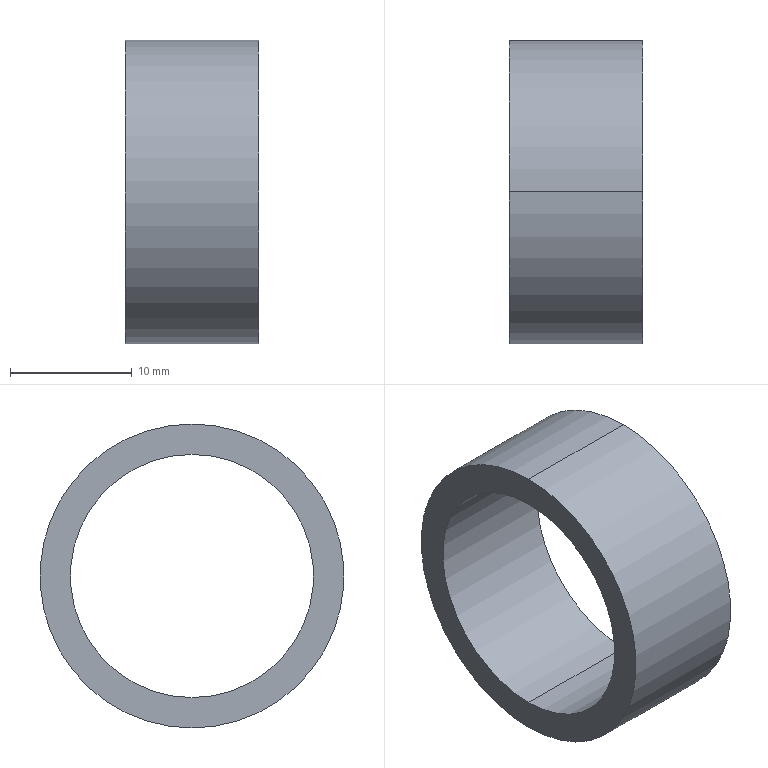Part | STEP file | 0244_Z_002_BSW20_2 | 1 solid | 6 faces | box 11 x 25 x 25 mm | volume 1944 mm3 | cylinder 4 | plane 2 | commonest cylinder face diameters 20 x2 25 x2
STEP:
#1=CARTESIAN_POINT('',(0.,0.,0.));
#2=DIRECTION('',(0.,0.,1.));
#3=DIRECTION('',(1.,0.,0.));
#4=AXIS2_PLACEMENT_3D('',#1,#2,#3);
#5=CARTESIAN_POINT('',(17.,30.,-12.5));
#6=VERTEX_POINT('',#5);
#7=CARTESIAN_POINT('',(17.,30.,12.5));
#8=VERTEX_POINT('',#7);
#9=CARTESIAN_POINT('',(17.,30.,0.));
#10=DIRECTION('',(1.,0.,0.));
#11=DIRECTION('',(0.,0.,-1.));
#12=AXIS2_PLACEMENT_3D('',#9,#10,#11);
#13=CIRCLE('',#12,12.5);
#14=CARTESIAN_POINT('',(22.5,30.,0.));
#15=DIRECTION('',(1.,0.,0.));
#16=DIRECTION('',(0.,0.,-1.));
#17=AXIS2_PLACEMENT_3D('',#14,#15,#16);
#18=CYLINDRICAL_SURFACE('',#17,12.5);
#19=CARTESIAN_POINT('',(0.,-5.5));
#20=DIRECTION('',(1.,0.));
#21=VECTOR('',#20,1.);
#22=LINE('',#19,#21);
#23=(GEOMETRIC_REPRESENTATION_CONTEXT(2)PARAMETRIC_REPRESENTATION_CONTEXT()REPRESENTATION_CONTEXT('',''));
#24=DEFINITIONAL_REPRESENTATION('',(#22),#23);
#25=PCURVE('',#18,#24);
#26=CARTESIAN_POINT('',(17.,18.75,0.));
#27=DIRECTION('',(-1.,0.,0.));
#28=DIRECTION('',(0.,0.,1.));
#29=AXIS2_PLACEMENT_3D('',#26,#27,#28);
#30=PLANE('',#29);
#31=CARTESIAN_POINT('',(-12.5,11.25));
#32=CARTESIAN_POINT('',(-12.5,32.901));
#33=CARTESIAN_POINT('',(6.25,22.075));
#34=CARTESIAN_POINT('',(25.,11.25));
#35=CARTESIAN_POINT('',(6.25,0.4247));
#36=CARTESIAN_POINT('',(-12.5,-10.401));
#37=CARTESIAN_POINT('',(-12.5,11.25));
#38=(BOUNDED_CURVE()B_SPLINE_CURVE(2,(#31,#32,#33,#34,#35,#36,#37),.UNSPECIFIED.,.T.,.F.)B_SPLINE_CURVE_WITH_KNOTS((1,2,2,2,2,1),(-2.094,0.,2.094,4.189,6.283,8.378),.UNSPECIFIED.)CURVE()GEOMETRIC_REPRESENTATION_ITEM()RATIONAL_B_SPLINE_CURVE((1.,0.5,1.,0.5,1.,0.5,1.))REPRESENTATION_ITEM(''));
#39=(GEOMETRIC_REPRESENTATION_CONTEXT(2)PARAMETRIC_REPRESENTATION_CONTEXT()REPRESENTATION_CONTEXT('',''));
#40=DEFINITIONAL_REPRESENTATION('',(#38),#39);
#41=PCURVE('',#30,#40);
#42=SURFACE_CURVE('',#13,(#25,#41),.PCURVE_S1.);
#43=EDGE_CURVE('',#6,#8,#42,.T.);
#44=ORIENTED_EDGE('',*,*,#43,.T.);
#45=CARTESIAN_POINT('',(28.,30.,12.5));
#46=VERTEX_POINT('',#45);
#47=CARTESIAN_POINT('',(22.5,30.,12.5));
#48=DIRECTION('',(1.,0.,0.));
#49=VECTOR('',#48,1.);
#50=LINE('',#47,#49);
#51=CARTESIAN_POINT('',(3.142,0.));
#52=DIRECTION('',(0.,1.));
#53=VECTOR('',#52,1.);
#54=LINE('',#51,#53);
#55=(GEOMETRIC_REPRESENTATION_CONTEXT(2)PARAMETRIC_REPRESENTATION_CONTEXT()REPRESENTATION_CONTEXT('',''));
#56=DEFINITIONAL_REPRESENTATION('',(#54),#55);
#57=PCURVE('',#18,#56);
#58=CARTESIAN_POINT('',(22.5,30.,0.));
#59=DIRECTION('',(1.,0.,0.));
#60=DIRECTION('',(0.,0.,-1.));
#61=AXIS2_PLACEMENT_3D('',#58,#59,#60);
#62=CYLINDRICAL_SURFACE('',#61,12.5);
#63=CARTESIAN_POINT('',(3.142,0.));
#64=DIRECTION('',(0.,1.));
#65=VECTOR('',#64,1.);
#66=LINE('',#63,#65);
#67=(GEOMETRIC_REPRESENTATION_CONTEXT(2)PARAMETRIC_REPRESENTATION_CONTEXT()REPRESENTATION_CONTEXT('',''));
#68=DEFINITIONAL_REPRESENTATION('',(#66),#67);
#69=PCURVE('',#62,#68);
#70=SURFACE_CURVE('',#50,(#57,#69),.PCURVE_S1.);
#71=EDGE_CURVE('',#8,#46,#70,.T.);
#72=ORIENTED_EDGE('',*,*,#71,.T.);
#73=CARTESIAN_POINT('',(28.,30.,-12.5));
#74=VERTEX_POINT('',#73);
#75=CARTESIAN_POINT('',(28.,30.,0.));
#76=DIRECTION('',(-1.,0.,0.));
#77=DIRECTION('',(0.,0.,-1.));
#78=AXIS2_PLACEMENT_3D('',#75,#76,#77);
#79=CIRCLE('',#78,12.5);
#80=CARTESIAN_POINT('',(6.283,5.5));
#81=DIRECTION('',(-1.,0.));
#82=VECTOR('',#81,1.);
#83=LINE('',#80,#82);
#84=(GEOMETRIC_REPRESENTATION_CONTEXT(2)PARAMETRIC_REPRESENTATION_CONTEXT()REPRESENTATION_CONTEXT('',''));
#85=DEFINITIONAL_REPRESENTATION('',(#83),#84);
#86=PCURVE('',#18,#85);
#87=CARTESIAN_POINT('',(28.,18.75,0.));
#88=DIRECTION('',(1.,0.,0.));
#89=DIRECTION('',(0.,0.,-1.));
#90=AXIS2_PLACEMENT_3D('',#87,#88,#89);
#91=PLANE('',#90);
#92=CARTESIAN_POINT('',(12.5,11.25));
#93=CARTESIAN_POINT('',(12.5,-10.401));
#94=CARTESIAN_POINT('',(-6.25,0.4247));
#95=CARTESIAN_POINT('',(-25.,11.25));
#96=CARTESIAN_POINT('',(-6.25,22.075));
#97=CARTESIAN_POINT('',(12.5,32.901));
#98=CARTESIAN_POINT('',(12.5,11.25));
#99=(BOUNDED_CURVE()B_SPLINE_CURVE(2,(#92,#93,#94,#95,#96,#97,#98),.UNSPECIFIED.,.T.,.F.)B_SPLINE_CURVE_WITH_KNOTS((1,2,2,2,2,1),(-2.094,0.,2.094,4.189,6.283,8.378),.UNSPECIFIED.)CURVE()GEOMETRIC_REPRESENTATION_ITEM()RATIONAL_B_SPLINE_CURVE((1.,0.5,1.,0.5,1.,0.5,1.))REPRESENTATION_ITEM(''));
#100=(GEOMETRIC_REPRESENTATION_CONTEXT(2)PARAMETRIC_REPRESENTATION_CONTEXT()REPRESENTATION_CONTEXT('',''));
#101=DEFINITIONAL_REPRESENTATION('',(#99),#100);
#102=PCURVE('',#91,#101);
#103=SURFACE_CURVE('',#79,(#86,#102),.PCURVE_S1.);
#104=EDGE_CURVE('',#46,#74,#103,.T.);
#105=ORIENTED_EDGE('',*,*,#104,.T.);
#106=CARTESIAN_POINT('',(22.5,30.,-12.5));
#107=DIRECTION('',(1.,0.,0.));
#108=VECTOR('',#107,1.);
#109=LINE('',#106,#108);
#110=CARTESIAN_POINT('',(0.,0.));
#111=DIRECTION('',(0.,1.));
#112=VECTOR('',#111,1.);
#113=LINE('',#110,#112);
#114=(GEOMETRIC_REPRESENTATION_CONTEXT(2)PARAMETRIC_REPRESENTATION_CONTEXT()REPRESENTATION_CONTEXT('',''));
#115=DEFINITIONAL_REPRESENTATION('',(#113),#114);
#116=PCURVE('',#18,#115);
#117=CARTESIAN_POINT('',(6.283,0.));
#118=DIRECTION('',(0.,1.));
#119=VECTOR('',#118,1.);
#120=LINE('',#117,#119);
#121=(GEOMETRIC_REPRESENTATION_CONTEXT(2)PARAMETRIC_REPRESENTATION_CONTEXT()REPRESENTATION_CONTEXT('',''));
#122=DEFINITIONAL_REPRESENTATION('',(#120),#121);
#123=PCURVE('',#62,#122);
#124=SURFACE_CURVE('',#109,(#116,#123),.PCURVE_S1.);
#125=EDGE_CURVE('',#6,#74,#124,.T.);
#126=ORIENTED_EDGE('',*,*,#125,.F.);
#127=EDGE_LOOP('',(#44,#72,#105,#126));
#128=FACE_BOUND('',#127,.T.);
#129=ADVANCED_FACE('',(#128),#18,.T.);
#130=CARTESIAN_POINT('',(17.,30.,-10.));
#131=VERTEX_POINT('',#130);
#132=CARTESIAN_POINT('',(28.,30.,-10.));
#133=VERTEX_POINT('',#132);
#134=CARTESIAN_POINT('',(22.5,30.,-10.));
#135=DIRECTION('',(1.,0.,0.));
#136=VECTOR('',#135,1.);
#137=LINE('',#134,#136);
#138=CARTESIAN_POINT('',(22.5,30.,0.));
#139=DIRECTION('',(1.,0.,0.));
#140=DIRECTION('',(0.,0.,-1.));
#141=AXIS2_PLACEMENT_3D('',#138,#139,#140);
#142=CYLINDRICAL_SURFACE('',#141,10.);
#143=CARTESIAN_POINT('',(6.283,0.));
#144=DIRECTION('',(0.,1.));
#145=VECTOR('',#144,1.);
#146=LINE('',#143,#145);
#147=(GEOMETRIC_REPRESENTATION_CONTEXT(2)PARAMETRIC_REPRESENTATION_CONTEXT()REPRESENTATION_CONTEXT('',''));
#148=DEFINITIONAL_REPRESENTATION('',(#146),#147);
#149=PCURVE('',#142,#148);
#150=CARTESIAN_POINT('',(22.5,30.,0.));
#151=DIRECTION('',(1.,0.,0.));
#152=DIRECTION('',(0.,0.,-1.));
#153=AXIS2_PLACEMENT_3D('',#150,#151,#152);
#154=CYLINDRICAL_SURFACE('',#153,10.);
#155=CARTESIAN_POINT('',(0.,0.));
#156=DIRECTION('',(0.,1.));
#157=VECTOR('',#156,1.);
#158=LINE('',#155,#157);
#159=(GEOMETRIC_REPRESENTATION_CONTEXT(2)PARAMETRIC_REPRESENTATION_CONTEXT()REPRESENTATION_CONTEXT('',''));
#160=DEFINITIONAL_REPRESENTATION('',(#158),#159);
#161=PCURVE('',#154,#160);
#162=SURFACE_CURVE('',#137,(#149,#161),.PCURVE_S1.);
#163=EDGE_CURVE('',#131,#133,#162,.T.);
#164=ORIENTED_EDGE('',*,*,#163,.T.);
#165=CARTESIAN_POINT('',(28.,30.,10.));
#166=VERTEX_POINT('',#165);
#167=CARTESIAN_POINT('',(28.,30.,0.));
#168=DIRECTION('',(-1.,0.,0.));
#169=DIRECTION('',(0.,0.,-1.));
#170=AXIS2_PLACEMENT_3D('',#167,#168,#169);
#171=CIRCLE('',#170,10.);
#172=CARTESIAN_POINT('',(6.283,5.5));
#173=DIRECTION('',(-1.,0.));
#174=VECTOR('',#173,1.);
#175=LINE('',#172,#174);
#176=(GEOMETRIC_REPRESENTATION_CONTEXT(2)PARAMETRIC_REPRESENTATION_CONTEXT()REPRESENTATION_CONTEXT('',''));
#177=DEFINITIONAL_REPRESENTATION('',(#175),#176);
#178=PCURVE('',#142,#177);
#179=CARTESIAN_POINT('',(10.,11.25));
#180=CARTESIAN_POINT('',(10.,-6.071));
#181=CARTESIAN_POINT('',(-5.,2.59));
#182=CARTESIAN_POINT('',(-20.,11.25));
#183=CARTESIAN_POINT('',(-5.,19.91));
#184=CARTESIAN_POINT('',(10.,28.571));
#185=CARTESIAN_POINT('',(10.,11.25));
#186=(BOUNDED_CURVE()B_SPLINE_CURVE(2,(#179,#180,#181,#182,#183,#184,#185),.UNSPECIFIED.,.T.,.F.)B_SPLINE_CURVE_WITH_KNOTS((1,2,2,2,2,1),(-2.094,0.,2.094,4.189,6.283,8.378),.UNSPECIFIED.)CURVE()GEOMETRIC_REPRESENTATION_ITEM()RATIONAL_B_SPLINE_CURVE((1.,0.5,1.,0.5,1.,0.5,1.))REPRESENTATION_ITEM(''));
#187=(GEOMETRIC_REPRESENTATION_CONTEXT(2)PARAMETRIC_REPRESENTATION_CONTEXT()REPRESENTATION_CONTEXT('',''));
#188=DEFINITIONAL_REPRESENTATION('',(#186),#187);
#189=PCURVE('',#91,#188);
#190=SURFACE_CURVE('',#171,(#178,#189),.PCURVE_S1.);
#191=EDGE_CURVE('',#133,#166,#190,.T.);
#192=ORIENTED_EDGE('',*,*,#191,.T.);
#193=CARTESIAN_POINT('',(17.,30.,10.));
#194=VERTEX_POINT('',#193);
#195=CARTESIAN_POINT('',(22.5,30.,10.));
#196=DIRECTION('',(1.,0.,0.));
#197=VECTOR('',#196,1.);
#198=LINE('',#195,#197);
#199=CARTESIAN_POINT('',(3.142,0.));
#200=DIRECTION('',(0.,1.));
#201=VECTOR('',#200,1.);
#202=LINE('',#199,#201);
#203=(GEOMETRIC_REPRESENTATION_CONTEXT(2)PARAMETRIC_REPRESENTATION_CONTEXT()REPRESENTATION_CONTEXT('',''));
#204=DEFINITIONAL_REPRESENTATION('',(#202),#203);
#205=PCURVE('',#142,#204);
#206=CARTESIAN_POINT('',(3.142,0.));
#207=DIRECTION('',(0.,1.));
#208=VECTOR('',#207,1.);
#209=LINE('',#206,#208);
#210=(GEOMETRIC_REPRESENTATION_CONTEXT(2)PARAMETRIC_REPRESENTATION_CONTEXT()REPRESENTATION_CONTEXT('',''));
#211=DEFINITIONAL_REPRESENTATION('',(#209),#210);
#212=PCURVE('',#154,#211);
#213=SURFACE_CURVE('',#198,(#205,#212),.PCURVE_S1.);
#214=EDGE_CURVE('',#194,#166,#213,.T.);
#215=ORIENTED_EDGE('',*,*,#214,.F.);
#216=CARTESIAN_POINT('',(17.,30.,0.));
#217=DIRECTION('',(1.,0.,0.));
#218=DIRECTION('',(0.,0.,-1.));
#219=AXIS2_PLACEMENT_3D('',#216,#217,#218);
#220=CIRCLE('',#219,10.);
#221=CARTESIAN_POINT('',(0.,-5.5));
#222=DIRECTION('',(1.,0.));
#223=VECTOR('',#222,1.);
#224=LINE('',#221,#223);
#225=(GEOMETRIC_REPRESENTATION_CONTEXT(2)PARAMETRIC_REPRESENTATION_CONTEXT()REPRESENTATION_CONTEXT('',''));
#226=DEFINITIONAL_REPRESENTATION('',(#224),#225);
#227=PCURVE('',#142,#226);
#228=CARTESIAN_POINT('',(-10.,11.25));
#229=CARTESIAN_POINT('',(-10.,28.571));
#230=CARTESIAN_POINT('',(5.,19.91));
#231=CARTESIAN_POINT('',(20.,11.25));
#232=CARTESIAN_POINT('',(5.,2.59));
#233=CARTESIAN_POINT('',(-10.,-6.071));
#234=CARTESIAN_POINT('',(-10.,11.25));
#235=(BOUNDED_CURVE()B_SPLINE_CURVE(2,(#228,#229,#230,#231,#232,#233,#234),.UNSPECIFIED.,.T.,.F.)B_SPLINE_CURVE_WITH_KNOTS((1,2,2,2,2,1),(-2.094,0.,2.094,4.189,6.283,8.378),.UNSPECIFIED.)CURVE()GEOMETRIC_REPRESENTATION_ITEM()RATIONAL_B_SPLINE_CURVE((1.,0.5,1.,0.5,1.,0.5,1.))REPRESENTATION_ITEM(''));
#236=(GEOMETRIC_REPRESENTATION_CONTEXT(2)PARAMETRIC_REPRESENTATION_CONTEXT()REPRESENTATION_CONTEXT('',''));
#237=DEFINITIONAL_REPRESENTATION('',(#235),#236);
#238=PCURVE('',#30,#237);
#239=SURFACE_CURVE('',#220,(#227,#238),.PCURVE_S1.);
#240=EDGE_CURVE('',#194,#131,#239,.T.);
#241=ORIENTED_EDGE('',*,*,#240,.T.);
#242=EDGE_LOOP('',(#164,#192,#215,#241));
#243=FACE_BOUND('',#242,.F.);
#244=ADVANCED_FACE('',(#243),#142,.F.);
#245=ORIENTED_EDGE('',*,*,#71,.F.);
#246=CARTESIAN_POINT('',(17.,30.,0.));
#247=DIRECTION('',(1.,0.,0.));
#248=DIRECTION('',(0.,0.,-1.));
#249=AXIS2_PLACEMENT_3D('',#246,#247,#248);
#250=CIRCLE('',#249,12.5);
#251=CARTESIAN_POINT('',(0.,-5.5));
#252=DIRECTION('',(1.,0.));
#253=VECTOR('',#252,1.);
#254=LINE('',#251,#253);
#255=(GEOMETRIC_REPRESENTATION_CONTEXT(2)PARAMETRIC_REPRESENTATION_CONTEXT()REPRESENTATION_CONTEXT('',''));
#256=DEFINITIONAL_REPRESENTATION('',(#254),#255);
#257=PCURVE('',#62,#256);
#258=CARTESIAN_POINT('',(-12.5,11.25));
#259=CARTESIAN_POINT('',(-12.5,32.901));
#260=CARTESIAN_POINT('',(6.25,22.075));
#261=CARTESIAN_POINT('',(25.,11.25));
#262=CARTESIAN_POINT('',(6.25,0.4247));
#263=CARTESIAN_POINT('',(-12.5,-10.401));
#264=CARTESIAN_POINT('',(-12.5,11.25));
#265=(BOUNDED_CURVE()B_SPLINE_CURVE(2,(#258,#259,#260,#261,#262,#263,#264),.UNSPECIFIED.,.T.,.F.)B_SPLINE_CURVE_WITH_KNOTS((1,2,2,2,2,1),(-2.094,0.,2.094,4.189,6.283,8.378),.UNSPECIFIED.)CURVE()GEOMETRIC_REPRESENTATION_ITEM()RATIONAL_B_SPLINE_CURVE((1.,0.5,1.,0.5,1.,0.5,1.))REPRESENTATION_ITEM(''));
#266=(GEOMETRIC_REPRESENTATION_CONTEXT(2)PARAMETRIC_REPRESENTATION_CONTEXT()REPRESENTATION_CONTEXT('',''));
#267=DEFINITIONAL_REPRESENTATION('',(#265),#266);
#268=PCURVE('',#30,#267);
#269=SURFACE_CURVE('',#250,(#257,#268),.PCURVE_S1.);
#270=EDGE_CURVE('',#8,#6,#269,.T.);
#271=ORIENTED_EDGE('',*,*,#270,.T.);
#272=ORIENTED_EDGE('',*,*,#125,.T.);
#273=CARTESIAN_POINT('',(28.,30.,0.));
#274=DIRECTION('',(-1.,0.,0.));
#275=DIRECTION('',(0.,0.,-1.));
#276=AXIS2_PLACEMENT_3D('',#273,#274,#275);
#277=CIRCLE('',#276,12.5);
#278=CARTESIAN_POINT('',(6.283,5.5));
#279=DIRECTION('',(-1.,0.));
#280=VECTOR('',#279,1.);
#281=LINE('',#278,#280);
#282=(GEOMETRIC_REPRESENTATION_CONTEXT(2)PARAMETRIC_REPRESENTATION_CONTEXT()REPRESENTATION_CONTEXT('',''));
#283=DEFINITIONAL_REPRESENTATION('',(#281),#282);
#284=PCURVE('',#62,#283);
#285=CARTESIAN_POINT('',(12.5,11.25));
#286=CARTESIAN_POINT('',(12.5,-10.401));
#287=CARTESIAN_POINT('',(-6.25,0.4247));
#288=CARTESIAN_POINT('',(-25.,11.25));
#289=CARTESIAN_POINT('',(-6.25,22.075));
#290=CARTESIAN_POINT('',(12.5,32.901));
#291=CARTESIAN_POINT('',(12.5,11.25));
#292=(BOUNDED_CURVE()B_SPLINE_CURVE(2,(#285,#286,#287,#288,#289,#290,#291),.UNSPECIFIED.,.T.,.F.)B_SPLINE_CURVE_WITH_KNOTS((1,2,2,2,2,1),(-2.094,0.,2.094,4.189,6.283,8.378),.UNSPECIFIED.)CURVE()GEOMETRIC_REPRESENTATION_ITEM()RATIONAL_B_SPLINE_CURVE((1.,0.5,1.,0.5,1.,0.5,1.))REPRESENTATION_ITEM(''));
#293=(GEOMETRIC_REPRESENTATION_CONTEXT(2)PARAMETRIC_REPRESENTATION_CONTEXT()REPRESENTATION_CONTEXT('',''));
#294=DEFINITIONAL_REPRESENTATION('',(#292),#293);
#295=PCURVE('',#91,#294);
#296=SURFACE_CURVE('',#277,(#284,#295),.PCURVE_S1.);
#297=EDGE_CURVE('',#74,#46,#296,.T.);
#298=ORIENTED_EDGE('',*,*,#297,.T.);
#299=EDGE_LOOP('',(#245,#271,#272,#298));
#300=FACE_BOUND('',#299,.T.);
#301=ADVANCED_FACE('',(#300),#62,.T.);
#302=ORIENTED_EDGE('',*,*,#43,.F.);
#303=ORIENTED_EDGE('',*,*,#270,.F.);
#304=EDGE_LOOP('',(#302,#303));
#305=FACE_BOUND('',#304,.T.);
#306=CARTESIAN_POINT('',(17.,30.,0.));
#307=DIRECTION('',(1.,0.,0.));
#308=DIRECTION('',(0.,0.,-1.));
#309=AXIS2_PLACEMENT_3D('',#306,#307,#308);
#310=CIRCLE('',#309,10.);
#311=CARTESIAN_POINT('',(-10.,11.25));
#312=CARTESIAN_POINT('',(-10.,28.571));
#313=CARTESIAN_POINT('',(5.,19.91));
#314=CARTESIAN_POINT('',(20.,11.25));
#315=CARTESIAN_POINT('',(5.,2.59));
#316=CARTESIAN_POINT('',(-10.,-6.071));
#317=CARTESIAN_POINT('',(-10.,11.25));
#318=(BOUNDED_CURVE()B_SPLINE_CURVE(2,(#311,#312,#313,#314,#315,#316,#317),.UNSPECIFIED.,.T.,.F.)B_SPLINE_CURVE_WITH_KNOTS((1,2,2,2,2,1),(-2.094,0.,2.094,4.189,6.283,8.378),.UNSPECIFIED.)CURVE()GEOMETRIC_REPRESENTATION_ITEM()RATIONAL_B_SPLINE_CURVE((1.,0.5,1.,0.5,1.,0.5,1.))REPRESENTATION_ITEM(''));
#319=(GEOMETRIC_REPRESENTATION_CONTEXT(2)PARAMETRIC_REPRESENTATION_CONTEXT()REPRESENTATION_CONTEXT('',''));
#320=DEFINITIONAL_REPRESENTATION('',(#318),#319);
#321=PCURVE('',#30,#320);
#322=CARTESIAN_POINT('',(0.,-5.5));
#323=DIRECTION('',(1.,0.));
#324=VECTOR('',#323,1.);
#325=LINE('',#322,#324);
#326=(GEOMETRIC_REPRESENTATION_CONTEXT(2)PARAMETRIC_REPRESENTATION_CONTEXT()REPRESENTATION_CONTEXT('',''));
#327=DEFINITIONAL_REPRESENTATION('',(#325),#326);
#328=PCURVE('',#154,#327);
#329=SURFACE_CURVE('',#310,(#321,#328),.PCURVE_S1.);
#330=EDGE_CURVE('',#131,#194,#329,.T.);
#331=ORIENTED_EDGE('',*,*,#330,.T.);
#332=ORIENTED_EDGE('',*,*,#240,.T.);
#333=EDGE_LOOP('',(#331,#332));
#334=FACE_BOUND('',#333,.T.);
#335=ADVANCED_FACE('',(#305,#334),#30,.T.);
#336=ORIENTED_EDGE('',*,*,#191,.T.);
#337=CARTESIAN_POINT('',(28.,30.,0.));
#338=DIRECTION('',(-1.,0.,0.));
#339=DIRECTION('',(0.,0.,-1.));
#340=AXIS2_PLACEMENT_3D('',#337,#338,#339);
#341=CIRCLE('',#340,10.);
#342=CARTESIAN_POINT('',(10.,11.25));
#343=CARTESIAN_POINT('',(10.,-6.071));
#344=CARTESIAN_POINT('',(-5.,2.59));
#345=CARTESIAN_POINT('',(-20.,11.25));
#346=CARTESIAN_POINT('',(-5.,19.91));
#347=CARTESIAN_POINT('',(10.,28.571));
#348=CARTESIAN_POINT('',(10.,11.25));
#349=(BOUNDED_CURVE()B_SPLINE_CURVE(2,(#342,#343,#344,#345,#346,#347,#348),.UNSPECIFIED.,.T.,.F.)B_SPLINE_CURVE_WITH_KNOTS((1,2,2,2,2,1),(-2.094,0.,2.094,4.189,6.283,8.378),.UNSPECIFIED.)CURVE()GEOMETRIC_REPRESENTATION_ITEM()RATIONAL_B_SPLINE_CURVE((1.,0.5,1.,0.5,1.,0.5,1.))REPRESENTATION_ITEM(''));
#350=(GEOMETRIC_REPRESENTATION_CONTEXT(2)PARAMETRIC_REPRESENTATION_CONTEXT()REPRESENTATION_CONTEXT('',''));
#351=DEFINITIONAL_REPRESENTATION('',(#349),#350);
#352=PCURVE('',#91,#351);
#353=CARTESIAN_POINT('',(6.283,5.5));
#354=DIRECTION('',(-1.,0.));
#355=VECTOR('',#354,1.);
#356=LINE('',#353,#355);
#357=(GEOMETRIC_REPRESENTATION_CONTEXT(2)PARAMETRIC_REPRESENTATION_CONTEXT()REPRESENTATION_CONTEXT('',''));
#358=DEFINITIONAL_REPRESENTATION('',(#356),#357);
#359=PCURVE('',#154,#358);
#360=SURFACE_CURVE('',#341,(#352,#359),.PCURVE_S1.);
#361=EDGE_CURVE('',#166,#133,#360,.T.);
#362=ORIENTED_EDGE('',*,*,#361,.T.);
#363=EDGE_LOOP('',(#336,#362));
#364=FACE_BOUND('',#363,.T.);
#365=ORIENTED_EDGE('',*,*,#297,.F.);
#366=ORIENTED_EDGE('',*,*,#104,.F.);
#367=EDGE_LOOP('',(#365,#366));
#368=FACE_BOUND('',#367,.T.);
#369=ADVANCED_FACE('',(#364,#368),#91,.T.);
#370=ORIENTED_EDGE('',*,*,#361,.T.);
#371=ORIENTED_EDGE('',*,*,#163,.F.);
#372=ORIENTED_EDGE('',*,*,#330,.T.);
#373=ORIENTED_EDGE('',*,*,#214,.T.);
#374=EDGE_LOOP('',(#370,#371,#372,#373));
#375=FACE_BOUND('',#374,.F.);
#376=ADVANCED_FACE('',(#375),#154,.F.);
#377=CLOSED_SHELL('',(#129,#244,#301,#335,#369,#376));
#378=MANIFOLD_SOLID_BREP('',#377);
#379=(LENGTH_UNIT()NAMED_UNIT(*)SI_UNIT(.MILLI.,.METRE.));
#380=UNCERTAINTY_MEASURE_WITH_UNIT(LENGTH_MEASURE(0.0000001),#379,'','');
#381=(NAMED_UNIT(*)PLANE_ANGLE_UNIT()SI_UNIT($,.RADIAN.));
#382=(NAMED_UNIT(*)SI_UNIT($,.STERADIAN.)SOLID_ANGLE_UNIT());
#383=(GEOMETRIC_REPRESENTATION_CONTEXT(3)GLOBAL_UNCERTAINTY_ASSIGNED_CONTEXT((#380))GLOBAL_UNIT_ASSIGNED_CONTEXT((#379,#381,#382))REPRESENTATION_CONTEXT('',''));
#384=ADVANCED_BREP_SHAPE_REPRESENTATION('',(#4,#378),#383);